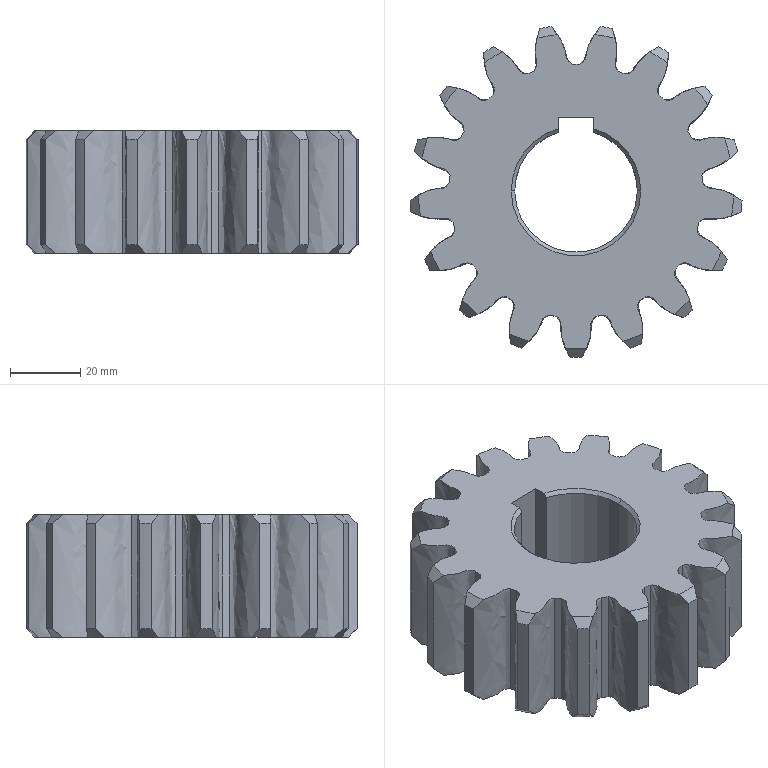Part | SolidWorks | features BaseBody 1 | 1 solid | 116 faces | box 94.845 x 94.471 x 35 mm | volume 159243 mm3 | cone 40 | cylinder 37 | spline 34 | plane 5 | commonest cylinder face diameters 72.5 x17 95 x17 35 x3